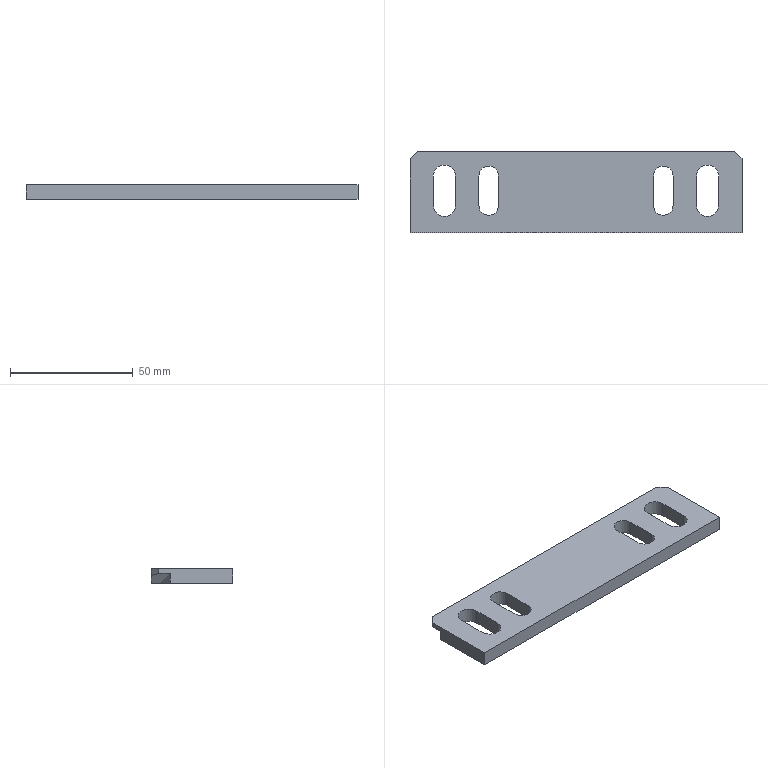Part | STEP file | gslz 2016.10.28-13_id1590_x_t | 1 solid | 29 faces | box 135 x 33 x 6 mm | volume 22607 mm3 | plane 21 | cylinder 8 | commonest cylinder face diameters 8 x4 9 x4